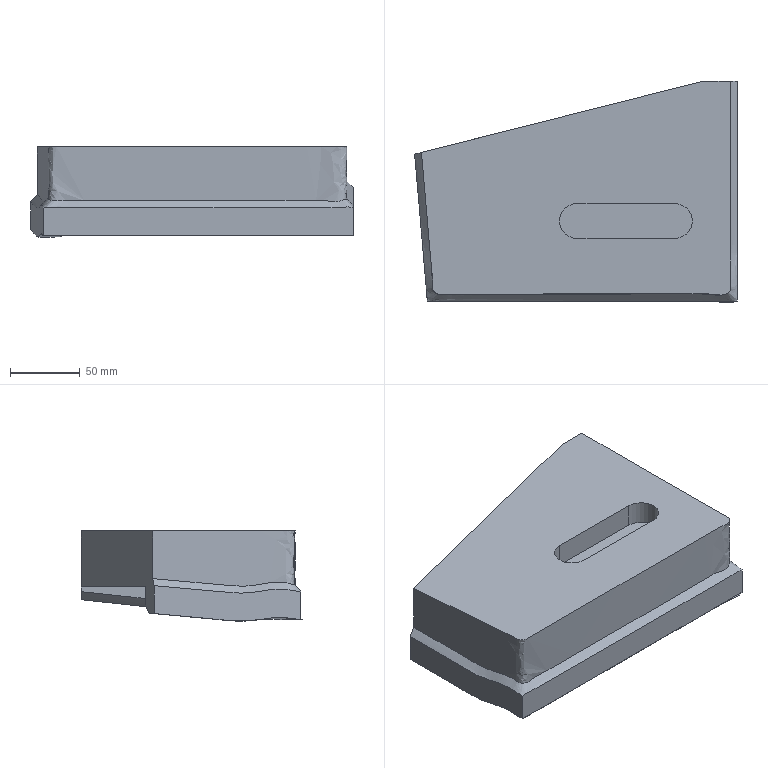Part | NX | features solid 2 | 1 solid | 36 faces | box 231.939 x 157.229 x 64.578 mm | volume 1093003 mm3 | spline 15 | plane 15 | cylinder 6 | commonest cylinder face diameters 30 x4 25 x2